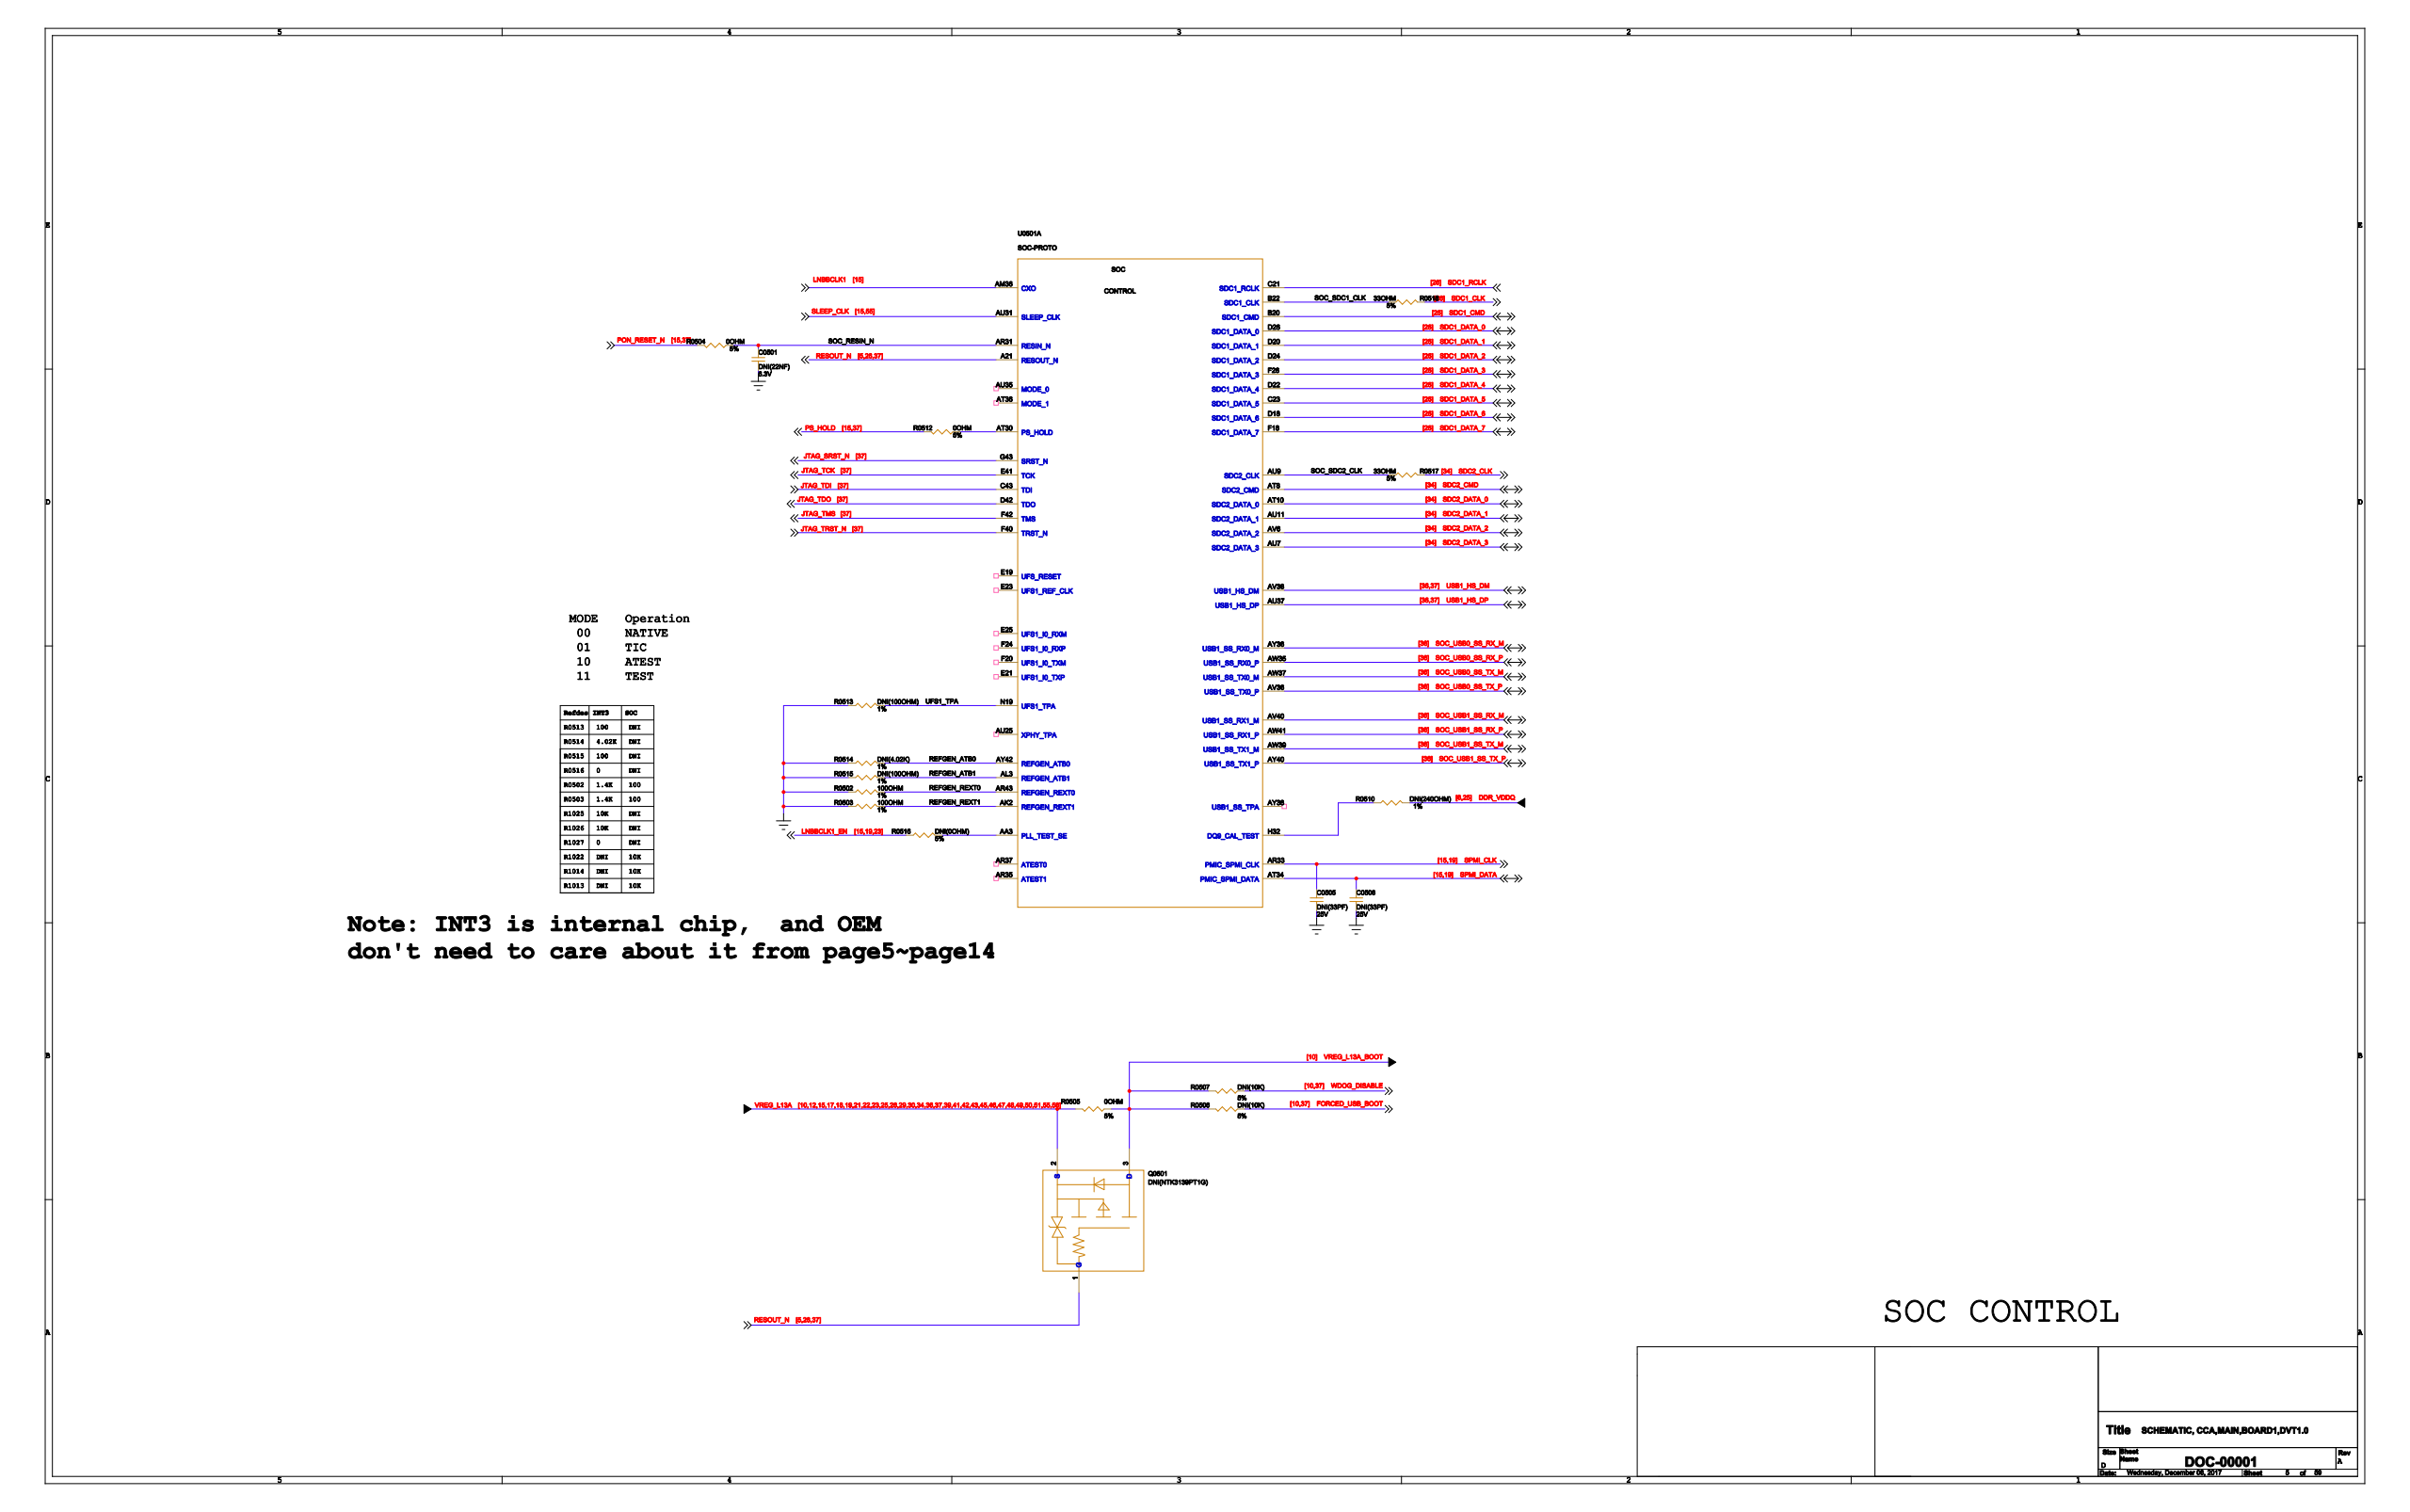Circuit board | KiCad | 1657 parts | 1365 nets | one sheet of the schematic
Parts on this sheet (reference | value | footprint):
C0501
C0505
C0506
Q0501
R0502
R0503
R0504
R0505
R0506
R0507
R0510
R0512
R0513
R0514
R0515
R0516
R0517
R0518
U0501
Nets of these parts (net: part-pin ...):
DDR_VDDQ: R0510-1
GND: C0501-2 C0505-2 C0506-2 R0502-2 R0503-2 R0513-2 R0514-2 R0515-2
RESOUT_N: Q0501-1 U0501-A21
VREG_L13A: Q0501-2 R0505-1
VREG_L13A_BOOT: Q0501-3 R0505-2 R0506-1 R0507-1
N23068124: R0516-1 U0501-AA3
LNBBCLK1_EN: R0516-2
SDC1_CMD: U0501-B20
SDC1_CLK: R0518-1
SOC_SDC1_CLK: R0518-2 U0501-B22
USB1_HS_DP: U0501-AU37
USB1_HS_DM: U0501-AV38
SDC2_DATA_3: U0501-AU7
SDC2_DATA_2: U0501-AV6
SDC1_DATA_0: U0501-D26
REFGEN_REXT1: R0503-1 U0501-AK2
SDC2_CMD: U0501-AT8
WDOG_DISABLE: R0507-2
N23025336: R0510-2 U0501-H32
SPMI_CLK: C0505-1 U0501-AR33
PON_RESET_N: R0504-1
SOC_RESIN_N: C0501-1 R0504-2 U0501-AR31
SLEEP_CLK: U0501-AU31
REFGEN_ATB0: R0514-1 U0501-AY42
REFGEN_ATB1: R0515-1 U0501-AL3
PS_HOLD: R0512-1
N22885505: R0512-2 U0501-AT30
SDC1_DATA_7: U0501-F18
SDC1_DATA_6: U0501-D18
SDC1_RCLK: U0501-C21
SDC1_DATA_1: U0501-D20
SDC1_DATA_4: U0501-D22
SDC1_DATA_2: U0501-D24
SDC1_DATA_5: U0501-C23
SDC1_DATA_3: U0501-F26
UFS1_TPA: R0513-1 U0501-N19
SDC2_DATA_1: U0501-AU11
SDC2_DATA_0: U0501-AT10
ORCED_USB_BOOT: R0506-2
LNBBCLK1: U0501-AM36
REFGEN_REXT0: R0502-1 U0501-AR43
SPMI_DATA: C0506-1 U0501-AT34
SOC_SDC2_CLK: R0517-2 U0501-AU9
JTAG_TDI: U0501-C43
JTAG_TDO: U0501-D42
JTAG_TCK: U0501-E41
JTAG_TRST_N: U0501-F40
JTAG_TMS: U0501-F42
JTAG_SRST_N: U0501-G43
SDC2_CLK: R0517-1